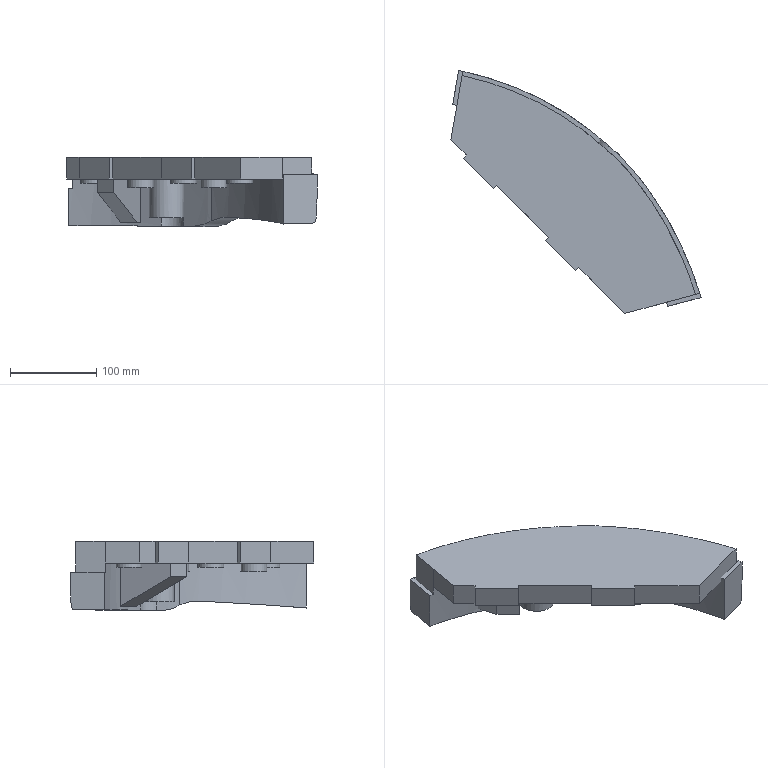Part | NX | features solid 2 | 1 solid | 66 faces | box 290.601 x 282.178 x 80.266 mm | volume 1797514 mm3 | spline 37 | plane 22 | cylinder 7 | commonest cylinder face diameters 30 x5 40 x2